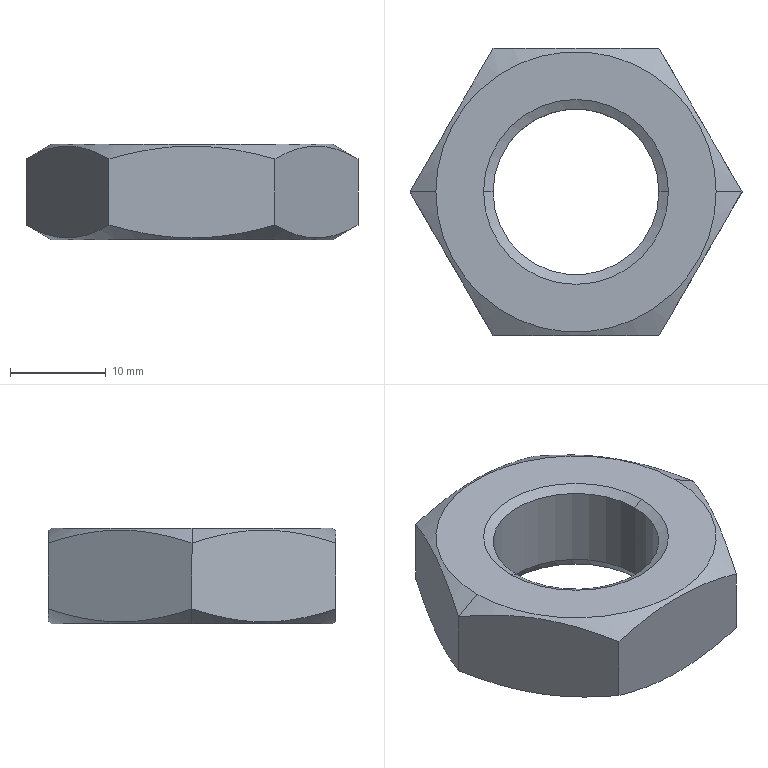Part | STEP file | Hex Thin Nut M20_GB_FASTENER_NUT_STNAB B M20-N | 1 solid | 18 faces | box 34.641 x 30 x 10 mm | volume 5315 mm3 | cone 8 | plane 8 | cylinder 2 | commonest cylinder face diameters 17.294 x2